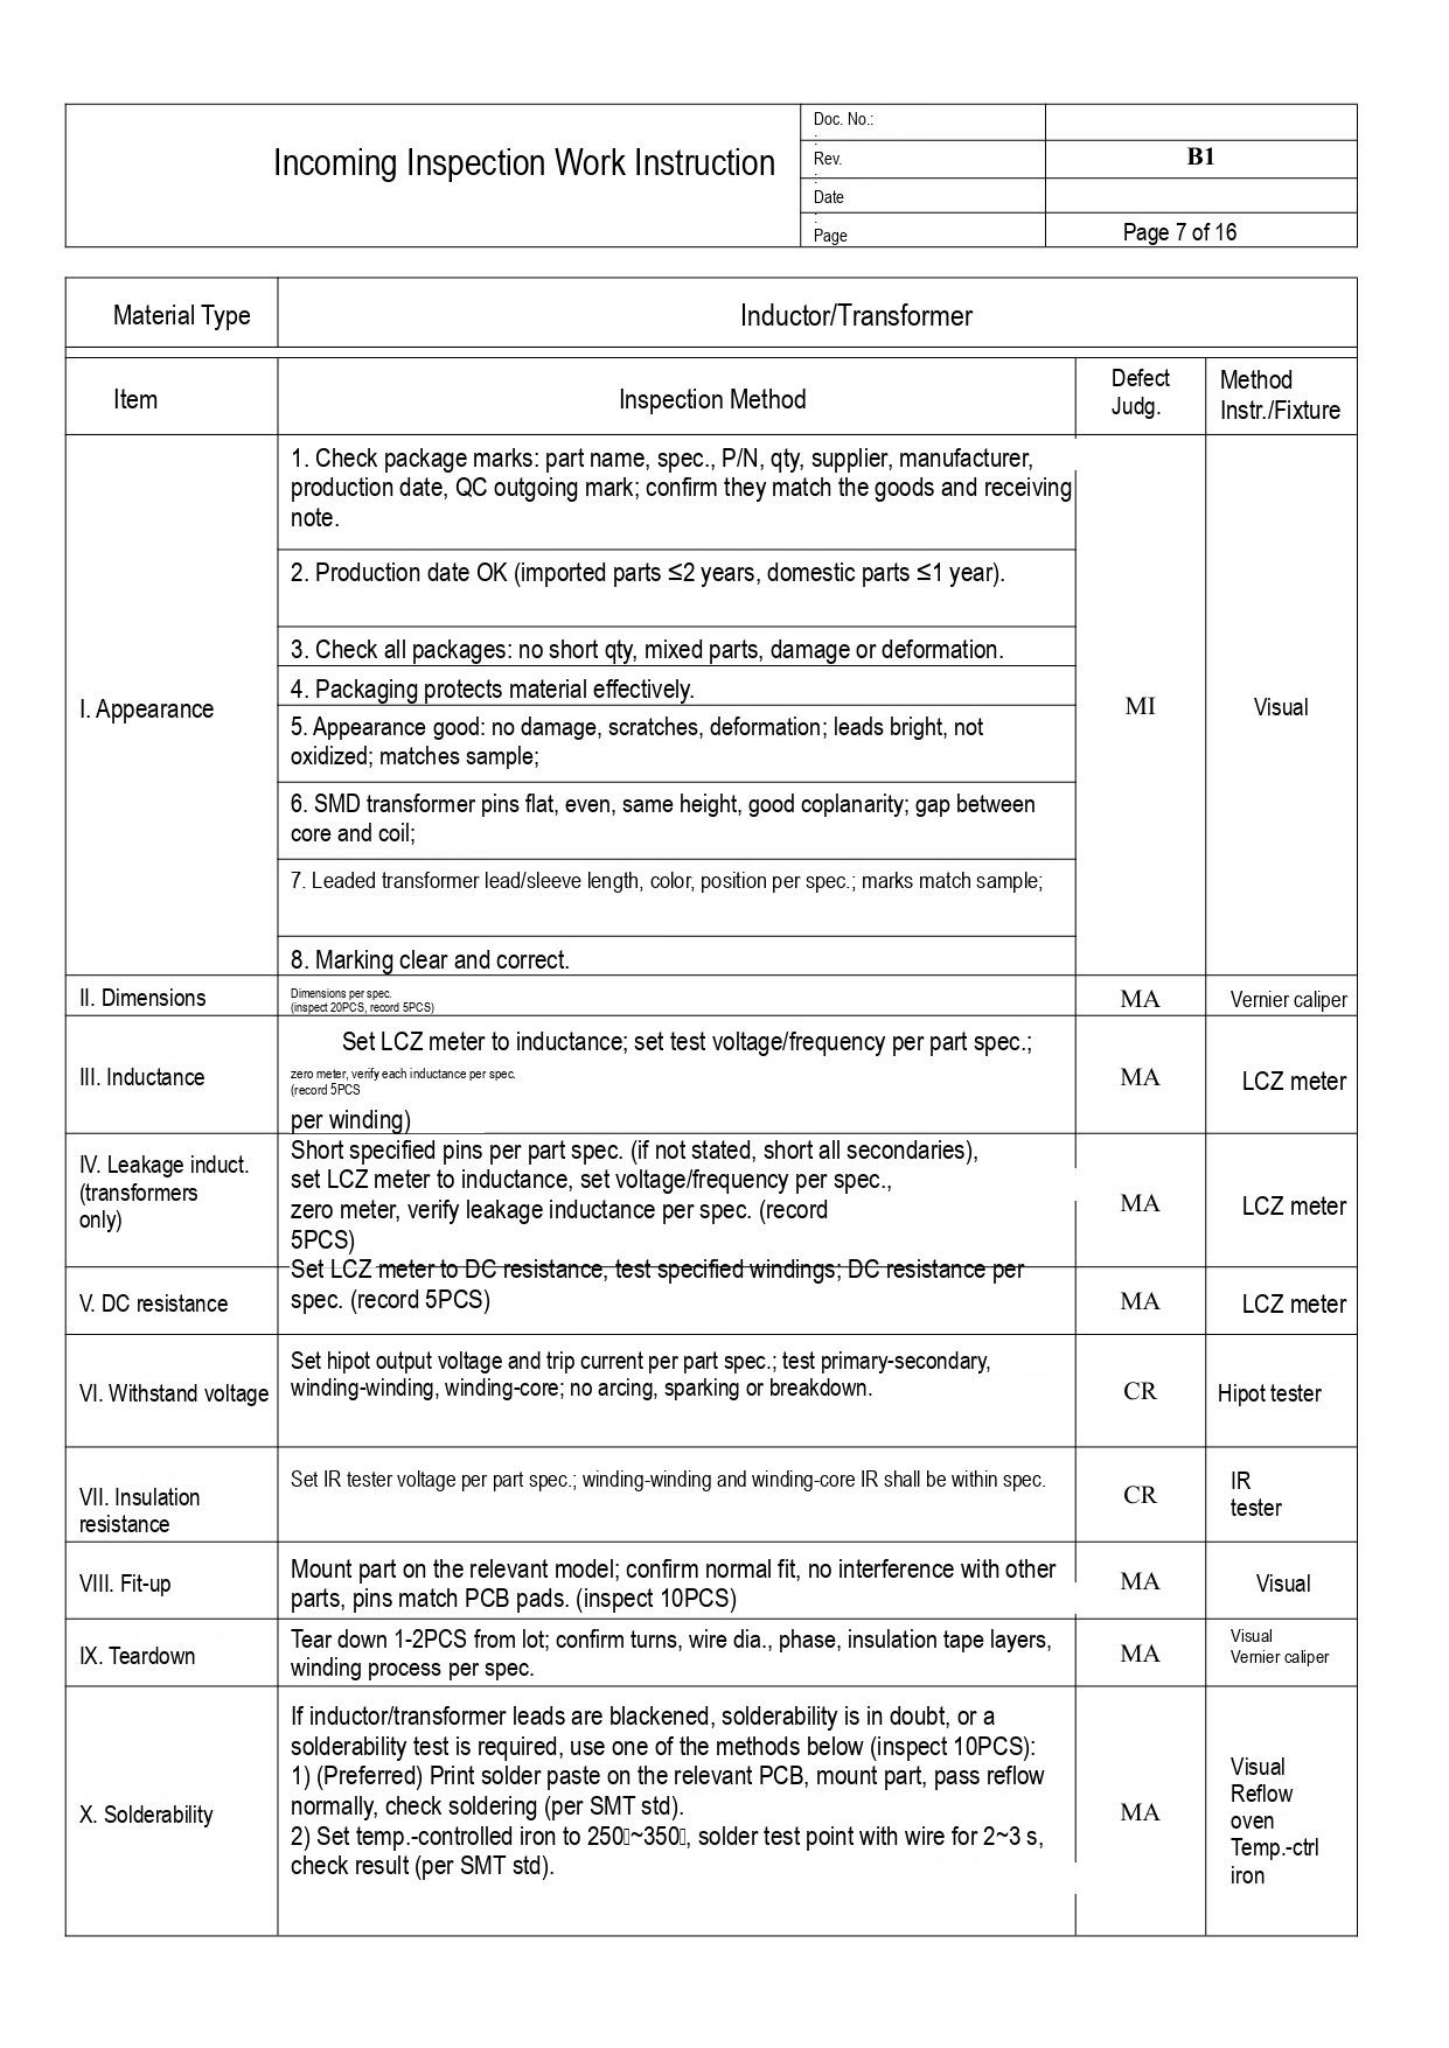# Incoming Inspection Work Instruction

| | |
|---|---|
| Doc. No.: | |
| Rev. | B1 |
| Date | |
| Page | Page 7 of 16 |

| Material Type | Inductor/Transformer | | |
|---|---|---|---|
| **Item** | **Inspection Method** | **Defect Judg.** | **Method Instr./Fixture** |
| I. Appearance | 1. Check package marks: part name, spec., P/N, qty, supplier, manufacturer, production date, QC outgoing mark; confirm they match the goods and receiving note. | MI | Visual |
| | 2. Production date OK (imported parts ≤2 years, domestic parts ≤1 year). | | |
| | 3. Check all packages: no short qty, mixed parts, damage or deformation. | | |
| | 4. Packaging protects material effectively. | | |
| | 5. Appearance good: no damage, scratches, deformation; leads bright, not oxidized; matches sample; | | |
| | 6. SMD transformer pins flat, even, same height, good coplanarity; gap between core and coil; | | |
| | 7. Leaded transformer lead/sleeve length, color, position per spec.; marks match sample; | | |
| | 8. Marking clear and correct. | | |
| II. Dimensions | Dimensions per spec. (inspect 20PCS, record 5PCS) | MA | Vernier caliper |
| III. Inductance | Set LCZ meter to inductance; set test voltage/frequency per part spec.; zero meter, verify each inductance per spec. (record 5PCS per winding) | MA | LCZ meter |
| IV. Leakage induct. (transformers only) | Short specified pins per part spec. (if not stated, short all secondaries), set LCZ meter to inductance, set voltage/frequency per spec., zero meter, verify leakage inductance per spec. (record 5PCS) | MA | LCZ meter |
| V. DC resistance | Set LCZ meter to DC resistance, test specified windings; DC resistance per spec. (record 5PCS) | MA | LCZ meter |
| VI. Withstand voltage | Set hipot output voltage and trip current per part spec.; test primary-secondary, winding-winding, winding-core; no arcing, sparking or breakdown. | CR | Hipot tester |
| VII. Insulation resistance | Set IR tester voltage per part spec.; winding-winding and winding-core IR shall be within spec. | CR | IR tester |
| VIII. Fit-up | Mount part on the relevant model; confirm normal fit, no interference with other parts, pins match PCB pads. (inspect 10PCS) | MA | Visual |
| IX. Teardown | Tear down 1-2PCS from lot; confirm turns, wire dia., phase, insulation tape layers, winding process per spec. | MA | Visual Vernier caliper |
| X. Solderability | If inductor/transformer leads are blackened, solderability is in doubt, or a solderability test is required, use one of the methods below (inspect 10PCS):<br>1) (Preferred) Print solder paste on the relevant PCB, mount part, pass reflow normally, check soldering (per SMT std).<br>2) Set temp.-controlled iron to 250~350, solder test point with wire for 2~3 s, check result (per SMT std). | MA | Visual Reflow oven Temp.-ctrl iron |
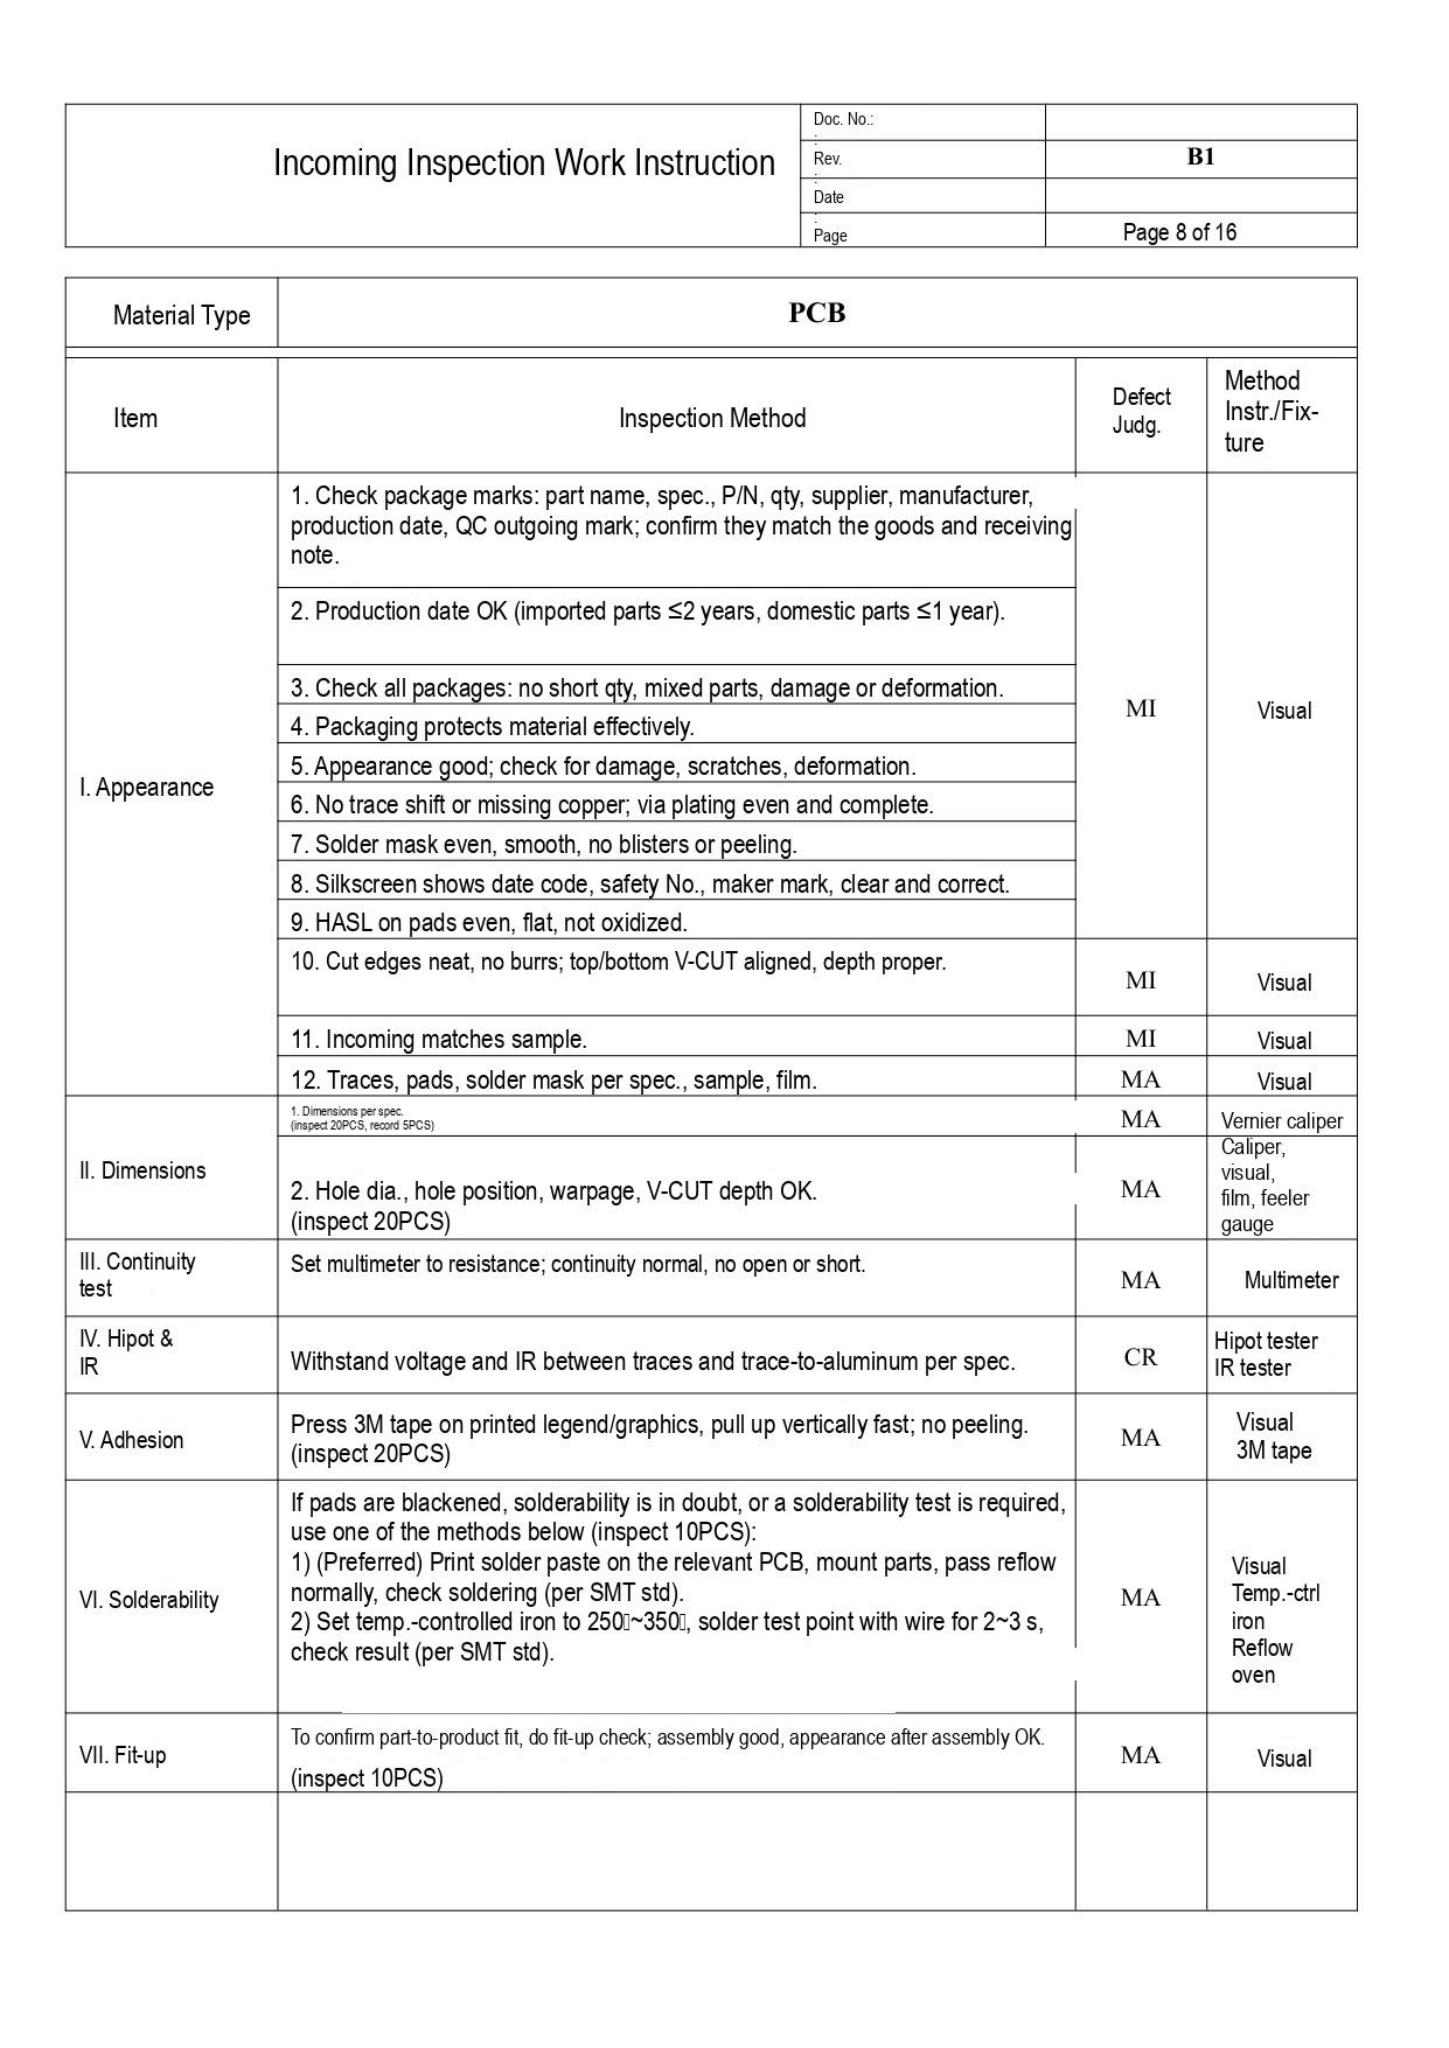**Incoming Inspection Work Instruction**

| Doc. No.: | |
|---|---|
| Rev. | B1 |
| Date | |
| Page | Page 8 of 16 |

| Material Type | PCB | | |
|---|---|---|---|

| Item | Inspection Method | Defect Judg. | Method Instr./Fix-ture |
|---|---|---|---|
| I. Appearance | 1. Check package marks: part name, spec., P/N, qty, supplier, manufacturer, production date, QC outgoing mark; confirm they match the goods and receiving note. | MI | Visual |
| | 2. Production date OK (imported parts ≤2 years, domestic parts ≤1 year). | | |
| | 3. Check all packages: no short qty, mixed parts, damage or deformation. | | |
| | 4. Packaging protects material effectively. | | |
| | 5. Appearance good; check for damage, scratches, deformation. | | |
| | 6. No trace shift or missing copper; via plating even and complete. | | |
| | 7. Solder mask even, smooth, no blisters or peeling. | | |
| | 8. Silkscreen shows date code, safety No., maker mark, clear and correct. | | |
| | 9. HASL on pads even, flat, not oxidized. | | |
| | 10. Cut edges neat, no burrs; top/bottom V-CUT aligned, depth proper. | MI | Visual |
| | 11. Incoming matches sample. | MI | Visual |
| | 12. Traces, pads, solder mask per spec., sample, film. | MA | Visual |
| II. Dimensions | 1. Dimensions per spec. (inspect 20PCS, record 5PCS) | MA | Vernier caliper |
| | 2. Hole dia., hole position, warpage, V-CUT depth OK. (inspect 20PCS) | MA | Caliper, visual, film, feeler gauge |
| III. Continuity test | Set multimeter to resistance; continuity normal, no open or short. | MA | Multimeter |
| IV. Hipot & IR | Withstand voltage and IR between traces and trace-to-aluminum per spec. | CR | Hipot tester IR tester |
| V. Adhesion | Press 3M tape on printed legend/graphics, pull up vertically fast; no peeling. (inspect 20PCS) | MA | Visual 3M tape |
| VI. Solderability | If pads are blackened, solderability is in doubt, or a solderability test is required, use one of the methods below (inspect 10PCS):<br>1) (Preferred) Print solder paste on the relevant PCB, mount parts, pass reflow normally, check soldering (per SMT std).<br>2) Set temp.-controlled iron to 250~350, solder test point with wire for 2~3 s, check result (per SMT std). | MA | Visual Temp.-ctrl iron Reflow oven |
| VII. Fit-up | To confirm part-to-product fit, do fit-up check; assembly good, appearance after assembly OK. (inspect 10PCS) | MA | Visual |
| | | | |
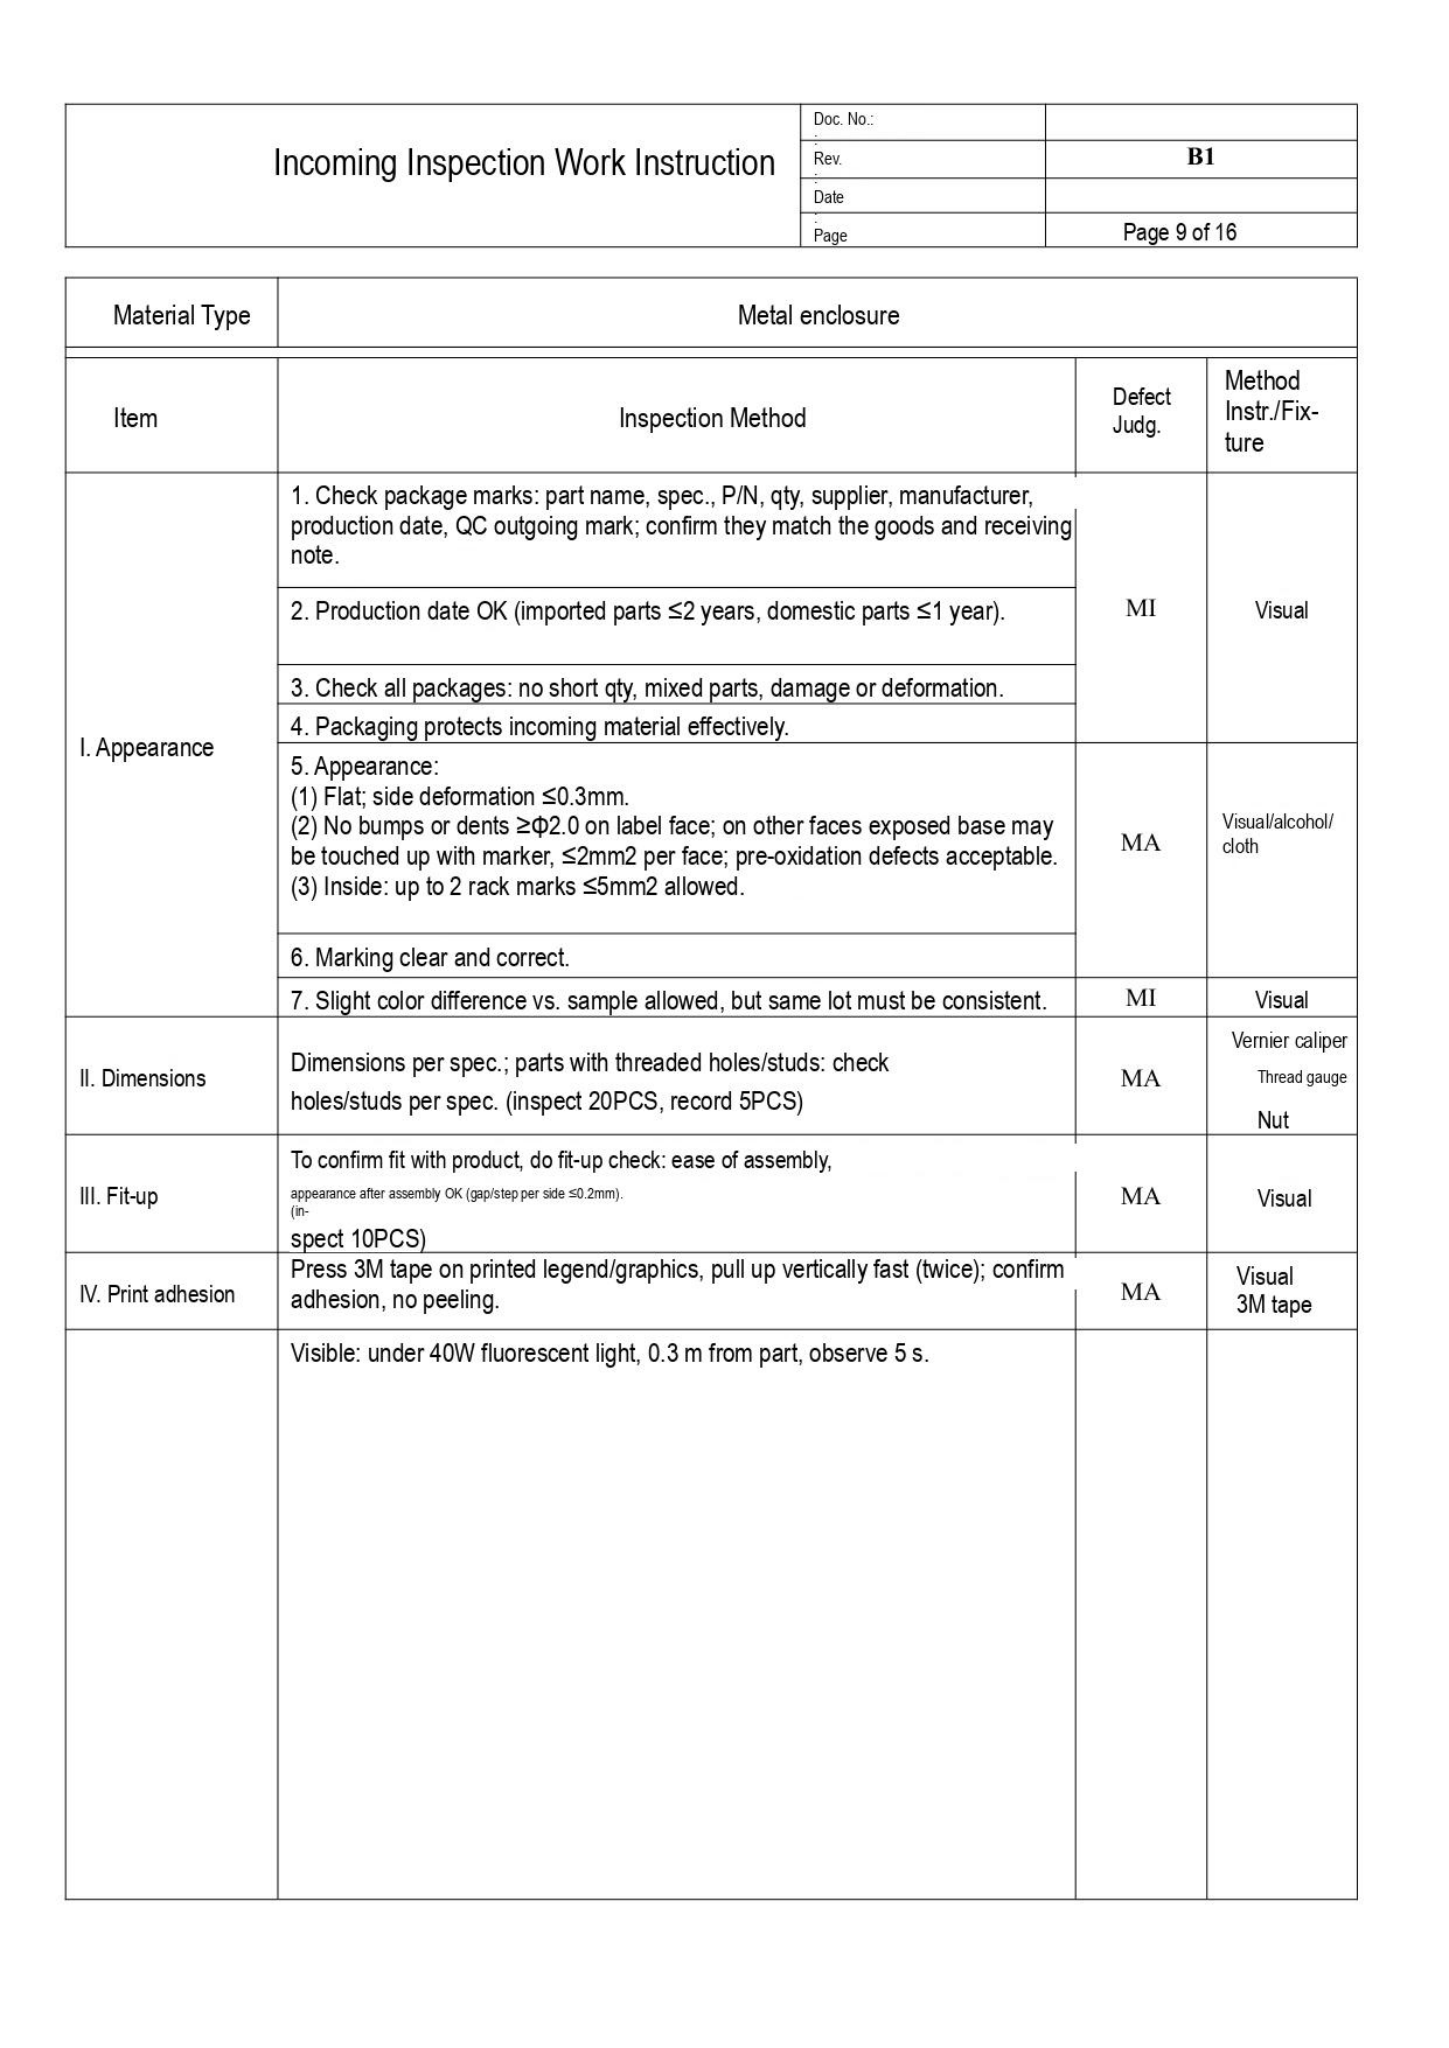Incoming Inspection Work Instruction

| Doc. No.: | |
|---|---|
| Rev. | B1 |
| Date | |
| Page | Page 9 of 16 |

| Material Type | Metal enclosure |
|---|---|

| Item | Inspection Method | Defect Judg. | Method Instr./Fix-ture |
|---|---|---|---|
| I. Appearance | 1. Check package marks: part name, spec., P/N, qty, supplier, manufacturer, production date, QC outgoing mark; confirm they match the goods and receiving note. | MI | Visual |
| | 2. Production date OK (imported parts ≤2 years, domestic parts ≤1 year). | | |
| | 3. Check all packages: no short qty, mixed parts, damage or deformation. | | |
| | 4. Packaging protects incoming material effectively. | | |
| | 5. Appearance:<br>(1) Flat; side deformation ≤0.3mm.<br>(2) No bumps or dents ≥Φ2.0 on label face; on other faces exposed base may be touched up with marker, ≤2mm2 per face; pre-oxidation defects acceptable.<br>(3) Inside: up to 2 rack marks ≤5mm2 allowed. | MA | Visual/alcohol/ cloth |
| | 6. Marking clear and correct. | | |
| | 7. Slight color difference vs. sample allowed, but same lot must be consistent. | MI | Visual |
| II. Dimensions | Dimensions per spec.; parts with threaded holes/studs: check holes/studs per spec. (inspect 20PCS, record 5PCS) | MA | Vernier caliper<br>Thread gauge<br>Nut |
| III. Fit-up | To confirm fit with product, do fit-up check: ease of assembly, appearance after assembly OK (gap/step per side ≤0.2mm). (in-spect 10PCS) | MA | Visual |
| IV. Print adhesion | Press 3M tape on printed legend/graphics, pull up vertically fast (twice); confirm adhesion, no peeling. | MA | Visual<br>3M tape |
| | Visible: under 40W fluorescent light, 0.3 m from part, observe 5 s. | | |
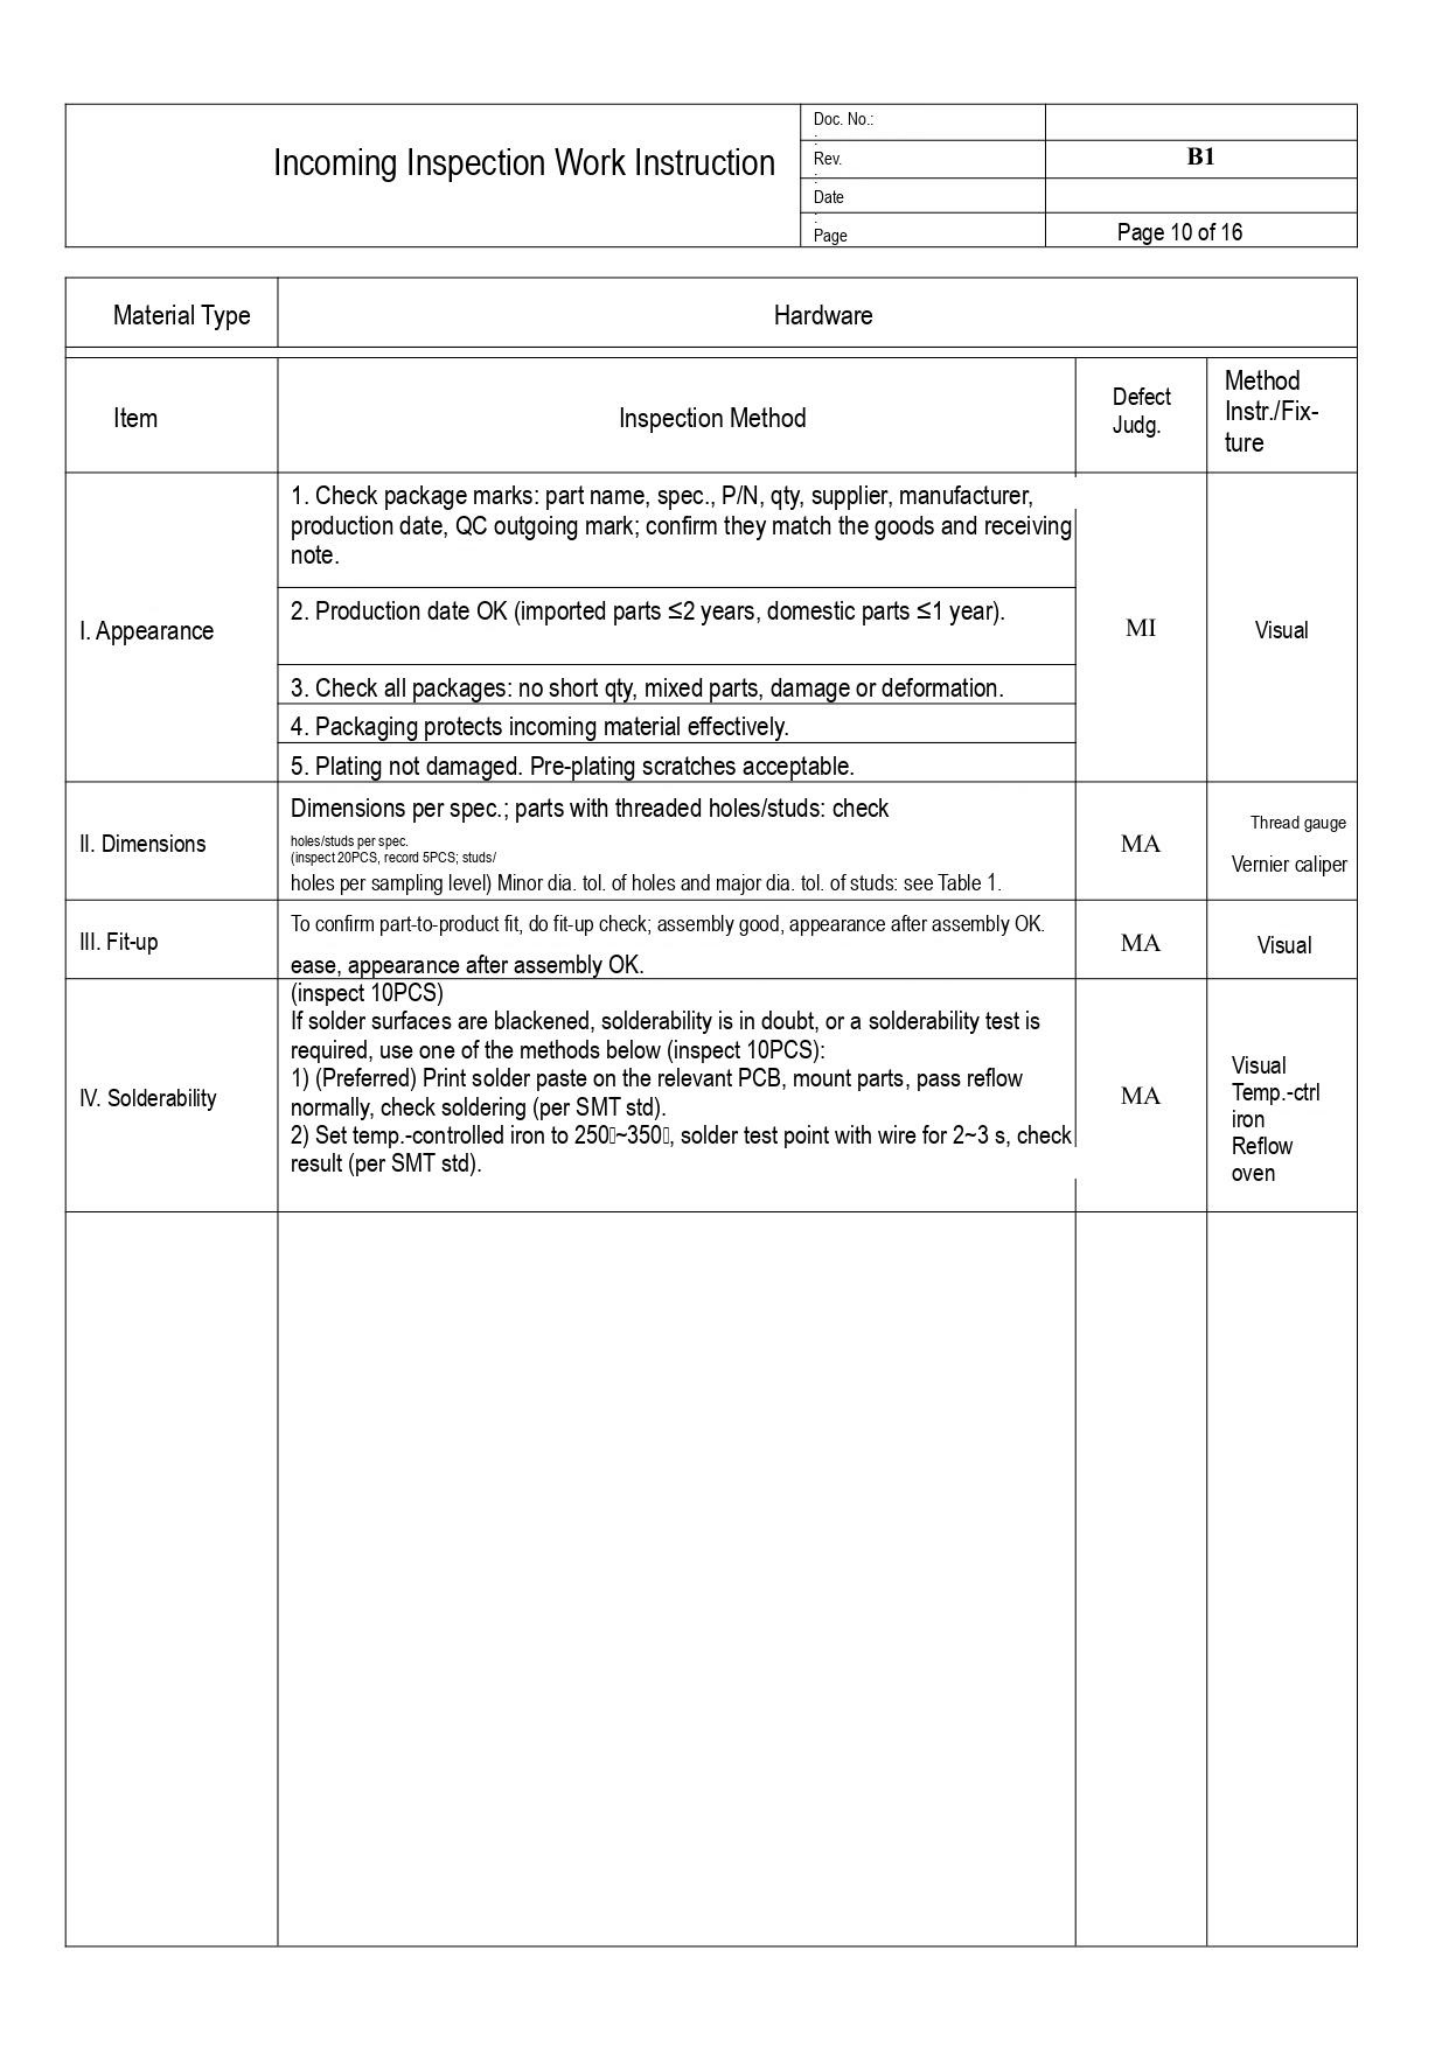Incoming Inspection Work Instruction

| Doc. No.: | |
|---|---|
| Rev. | B1 |
| Date | |
| Page | Page 10 of 16 |

| Material Type | Hardware |
|---|---|

| Item | Inspection Method | Defect Judg. | Method Instr./Fix-ture |
|---|---|---|---|
| I. Appearance | 1. Check package marks: part name, spec., P/N, qty, supplier, manufacturer, production date, QC outgoing mark; confirm they match the goods and receiving note. | MI | Visual |
| | 2. Production date OK (imported parts ≤2 years, domestic parts ≤1 year). | | |
| | 3. Check all packages: no short qty, mixed parts, damage or deformation. | | |
| | 4. Packaging protects incoming material effectively. | | |
| | 5. Plating not damaged. Pre-plating scratches acceptable. | | |
| II. Dimensions | Dimensions per spec.; parts with threaded holes/studs: check holes/studs per spec. (inspect 20PCS, record 5PCS; studs/ holes per sampling level) Minor dia. tol. of holes and major dia. tol. of studs: see Table 1. | MA | Thread gauge Vernier caliper |
| III. Fit-up | To confirm part-to-product fit, do fit-up check; assembly good, appearance after assembly OK. ease, appearance after assembly OK. | MA | Visual |
| IV. Solderability | (inspect 10PCS) If solder surfaces are blackened, solderability is in doubt, or a solderability test is required, use one of the methods below (inspect 10PCS): 1) (Preferred) Print solder paste on the relevant PCB, mount parts, pass reflow normally, check soldering (per SMT std). 2) Set temp.-controlled iron to 250~350, solder test point with wire for 2~3 s, check result (per SMT std). | MA | Visual Temp.-ctrl iron Reflow oven |
| | | | |
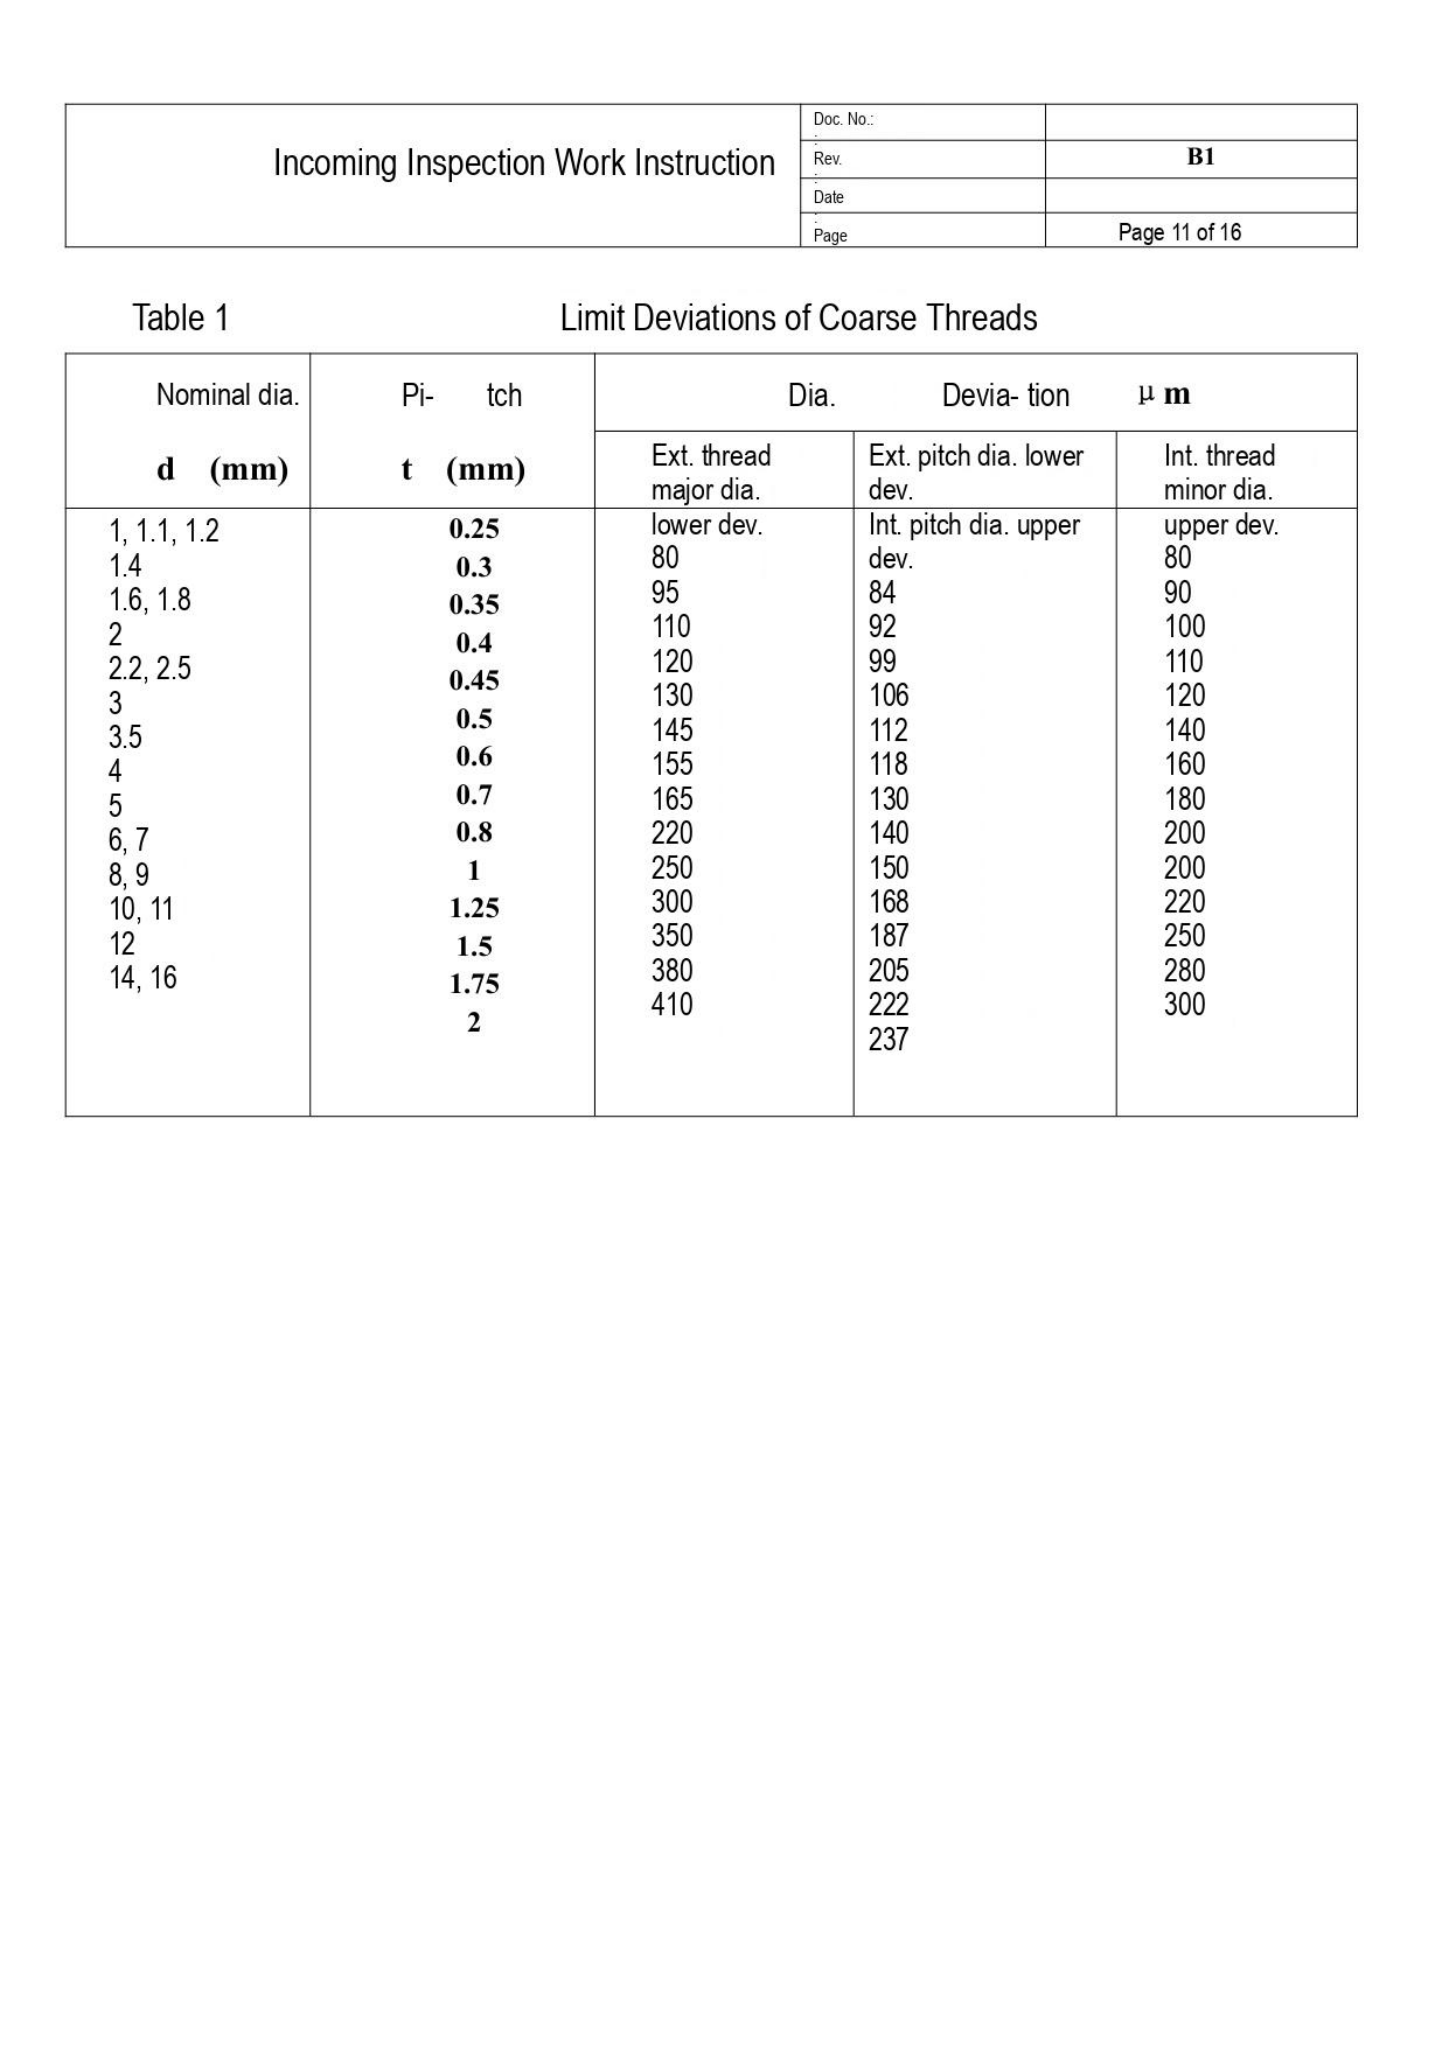| Incoming Inspection Work Instruction | Doc. No.: | |
|---|---|---|
| | Rev. | B1 |
| | Date | |
| | Page | Page 11 of 16 |

Table 1 Limit Deviations of Coarse Threads

| Nominal dia.<br>d (mm) | Pi- tch<br>t (mm) | Dia. Devia- tion μm<br>Ext. thread major dia. | Dia. Devia- tion μm<br>Ext. pitch dia. lower dev. | Dia. Devia- tion μm<br>Int. thread minor dia. |
|---|---|---|---|---|
| 1, 1.1, 1.2<br>1.4<br>1.6, 1.8<br>2<br>2.2, 2.5<br>3<br>3.5<br>4<br>5<br>6, 7<br>8, 9<br>10, 11<br>12<br>14, 16 | 0.25<br>0.3<br>0.35<br>0.4<br>0.45<br>0.5<br>0.6<br>0.7<br>0.8<br>1<br>1.25<br>1.5<br>1.75<br>2 | lower dev.<br>80<br>95<br>110<br>120<br>130<br>145<br>155<br>165<br>220<br>250<br>300<br>350<br>380<br>410 | Int. pitch dia. upper dev.<br>84<br>92<br>99<br>106<br>112<br>118<br>130<br>140<br>150<br>168<br>187<br>205<br>222<br>237 | upper dev.<br>80<br>90<br>100<br>110<br>120<br>140<br>160<br>180<br>200<br>200<br>220<br>250<br>280<br>300 |
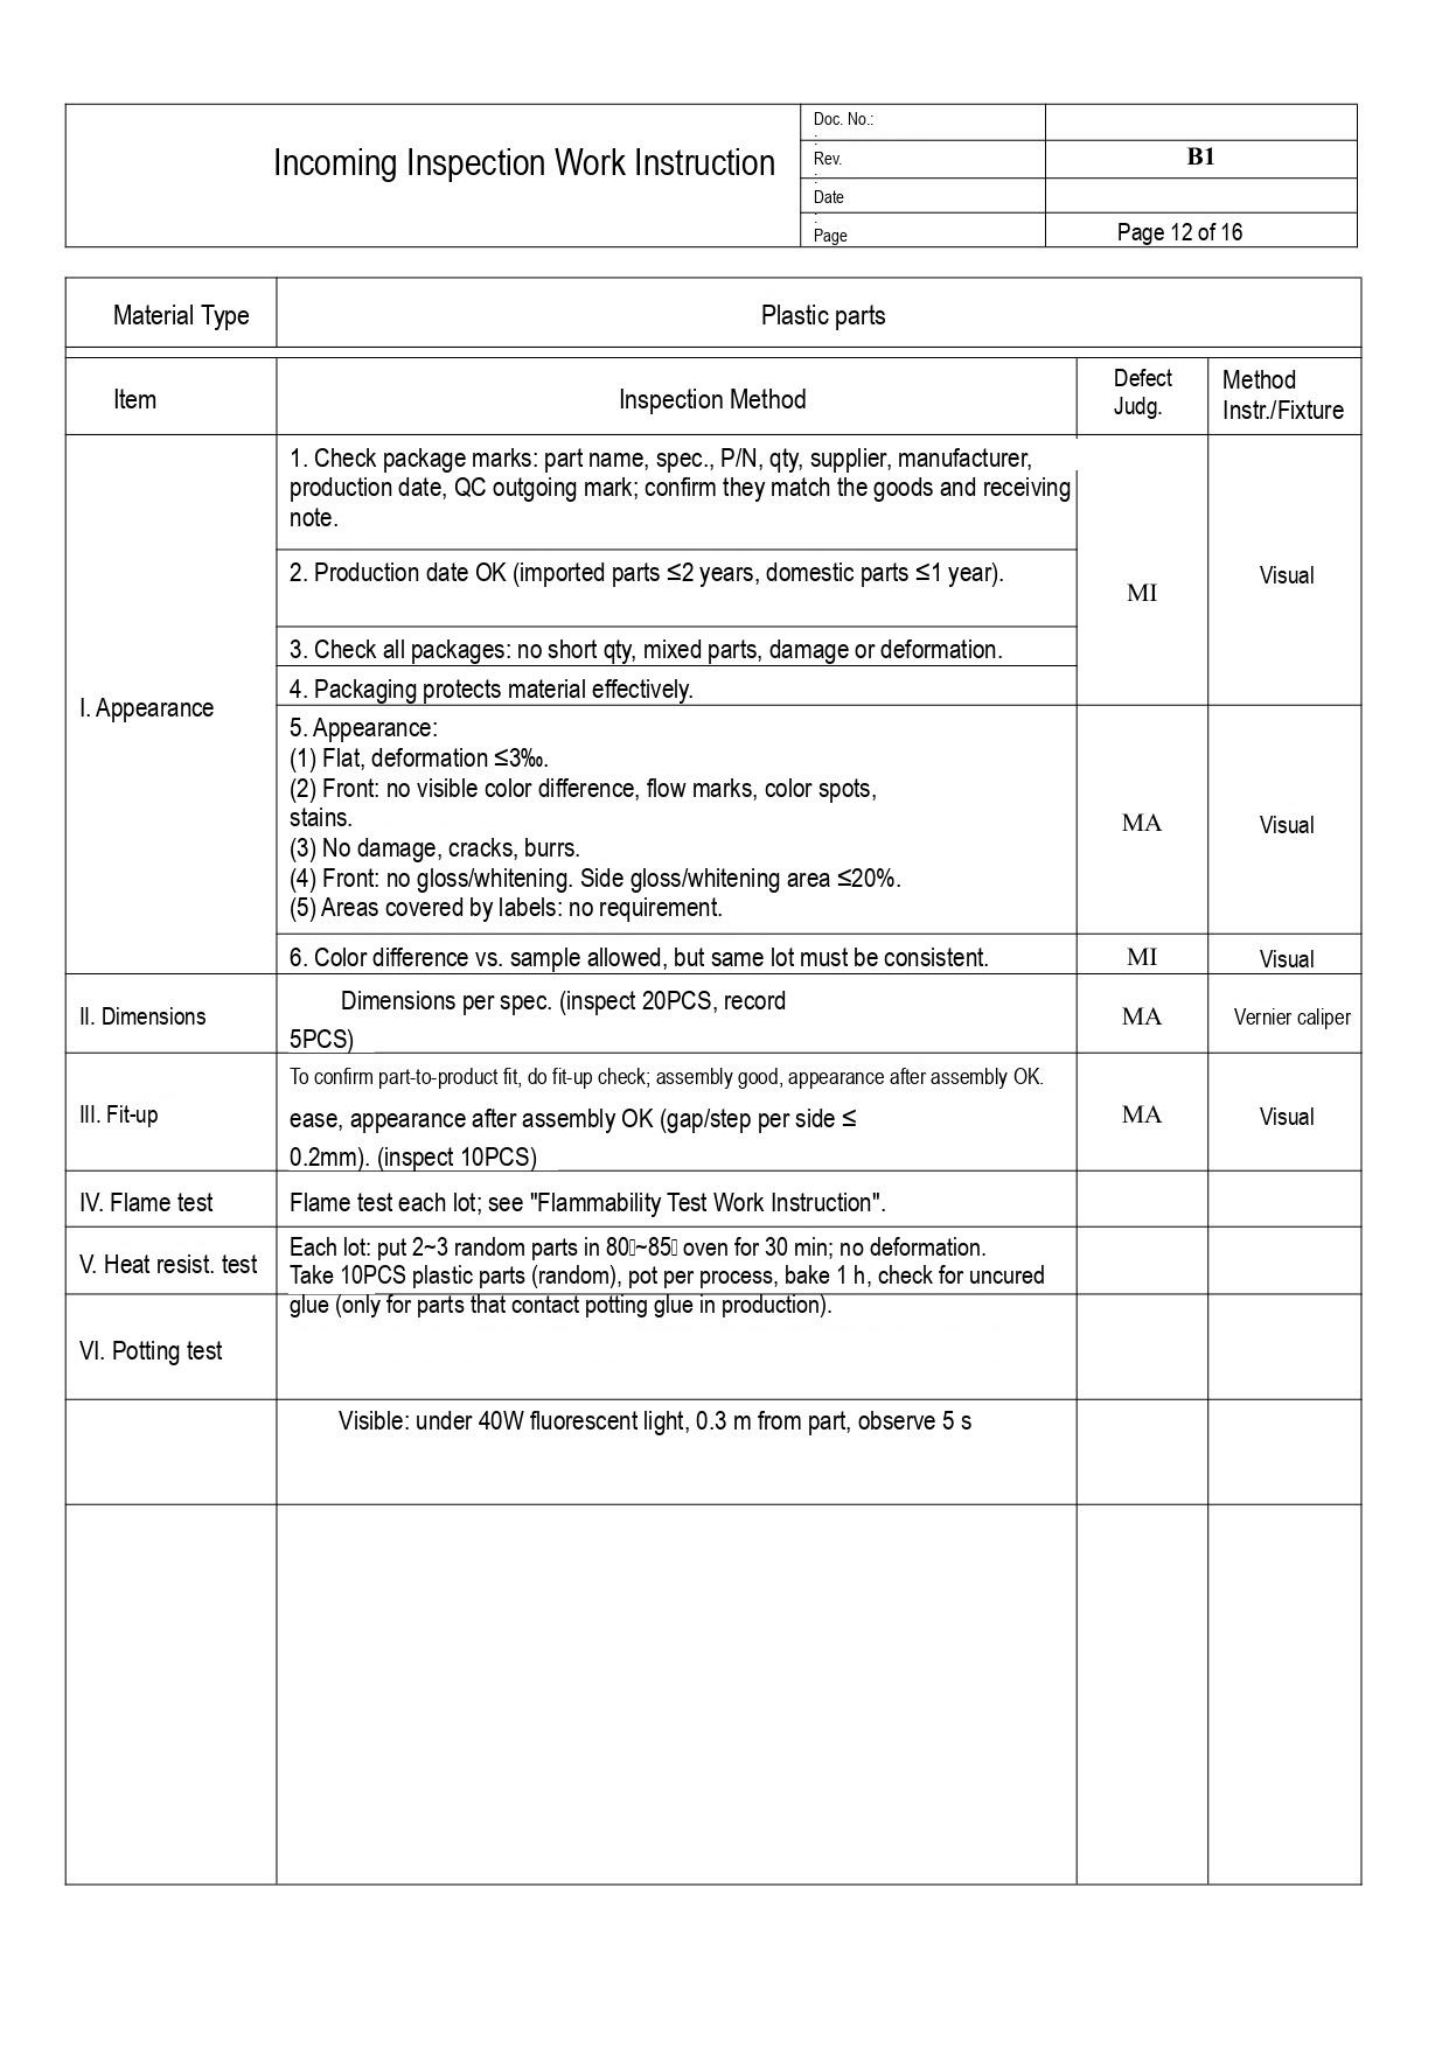# Incoming Inspection Work Instruction

| Doc. No.: | |
|---|---|
| Rev. | B1 |
| Date | |
| Page | Page 12 of 16 |

| Material Type | Plastic parts | | |
|---|---|---|---|
| **Item** | **Inspection Method** | **Defect Judg.** | **Method Instr./Fixture** |
| I. Appearance | 1. Check package marks: part name, spec., P/N, qty, supplier, manufacturer, production date, QC outgoing mark; confirm they match the goods and receiving note. | MI | Visual |
| | 2. Production date OK (imported parts ≤2 years, domestic parts ≤1 year). | | |
| | 3. Check all packages: no short qty, mixed parts, damage or deformation. | | |
| | 4. Packaging protects material effectively. | | |
| | 5. Appearance:<br>(1) Flat, deformation ≤3‰.<br>(2) Front: no visible color difference, flow marks, color spots, stains.<br>(3) No damage, cracks, burrs.<br>(4) Front: no gloss/whitening. Side gloss/whitening area ≤20%.<br>(5) Areas covered by labels: no requirement. | MA | Visual |
| | 6. Color difference vs. sample allowed, but same lot must be consistent. | MI | Visual |
| II. Dimensions | Dimensions per spec. (inspect 20PCS, record 5PCS) | MA | Vernier caliper |
| III. Fit-up | To confirm part-to-product fit, do fit-up check; assembly good, appearance after assembly OK.<br>ease, appearance after assembly OK (gap/step per side ≤ 0.2mm). (inspect 10PCS) | MA | Visual |
| IV. Flame test | Flame test each lot; see "Flammability Test Work Instruction". | | |
| V. Heat resist. test | Each lot: put 2~3 random parts in 80~85 oven for 30 min; no deformation. | | |
| VI. Potting test | Take 10PCS plastic parts (random), pot per process, bake 1 h, check for uncured glue (only for parts that contact potting glue in production). | | |
| | Visible: under 40W fluorescent light, 0.3 m from part, observe 5 s | | |
| | | | |